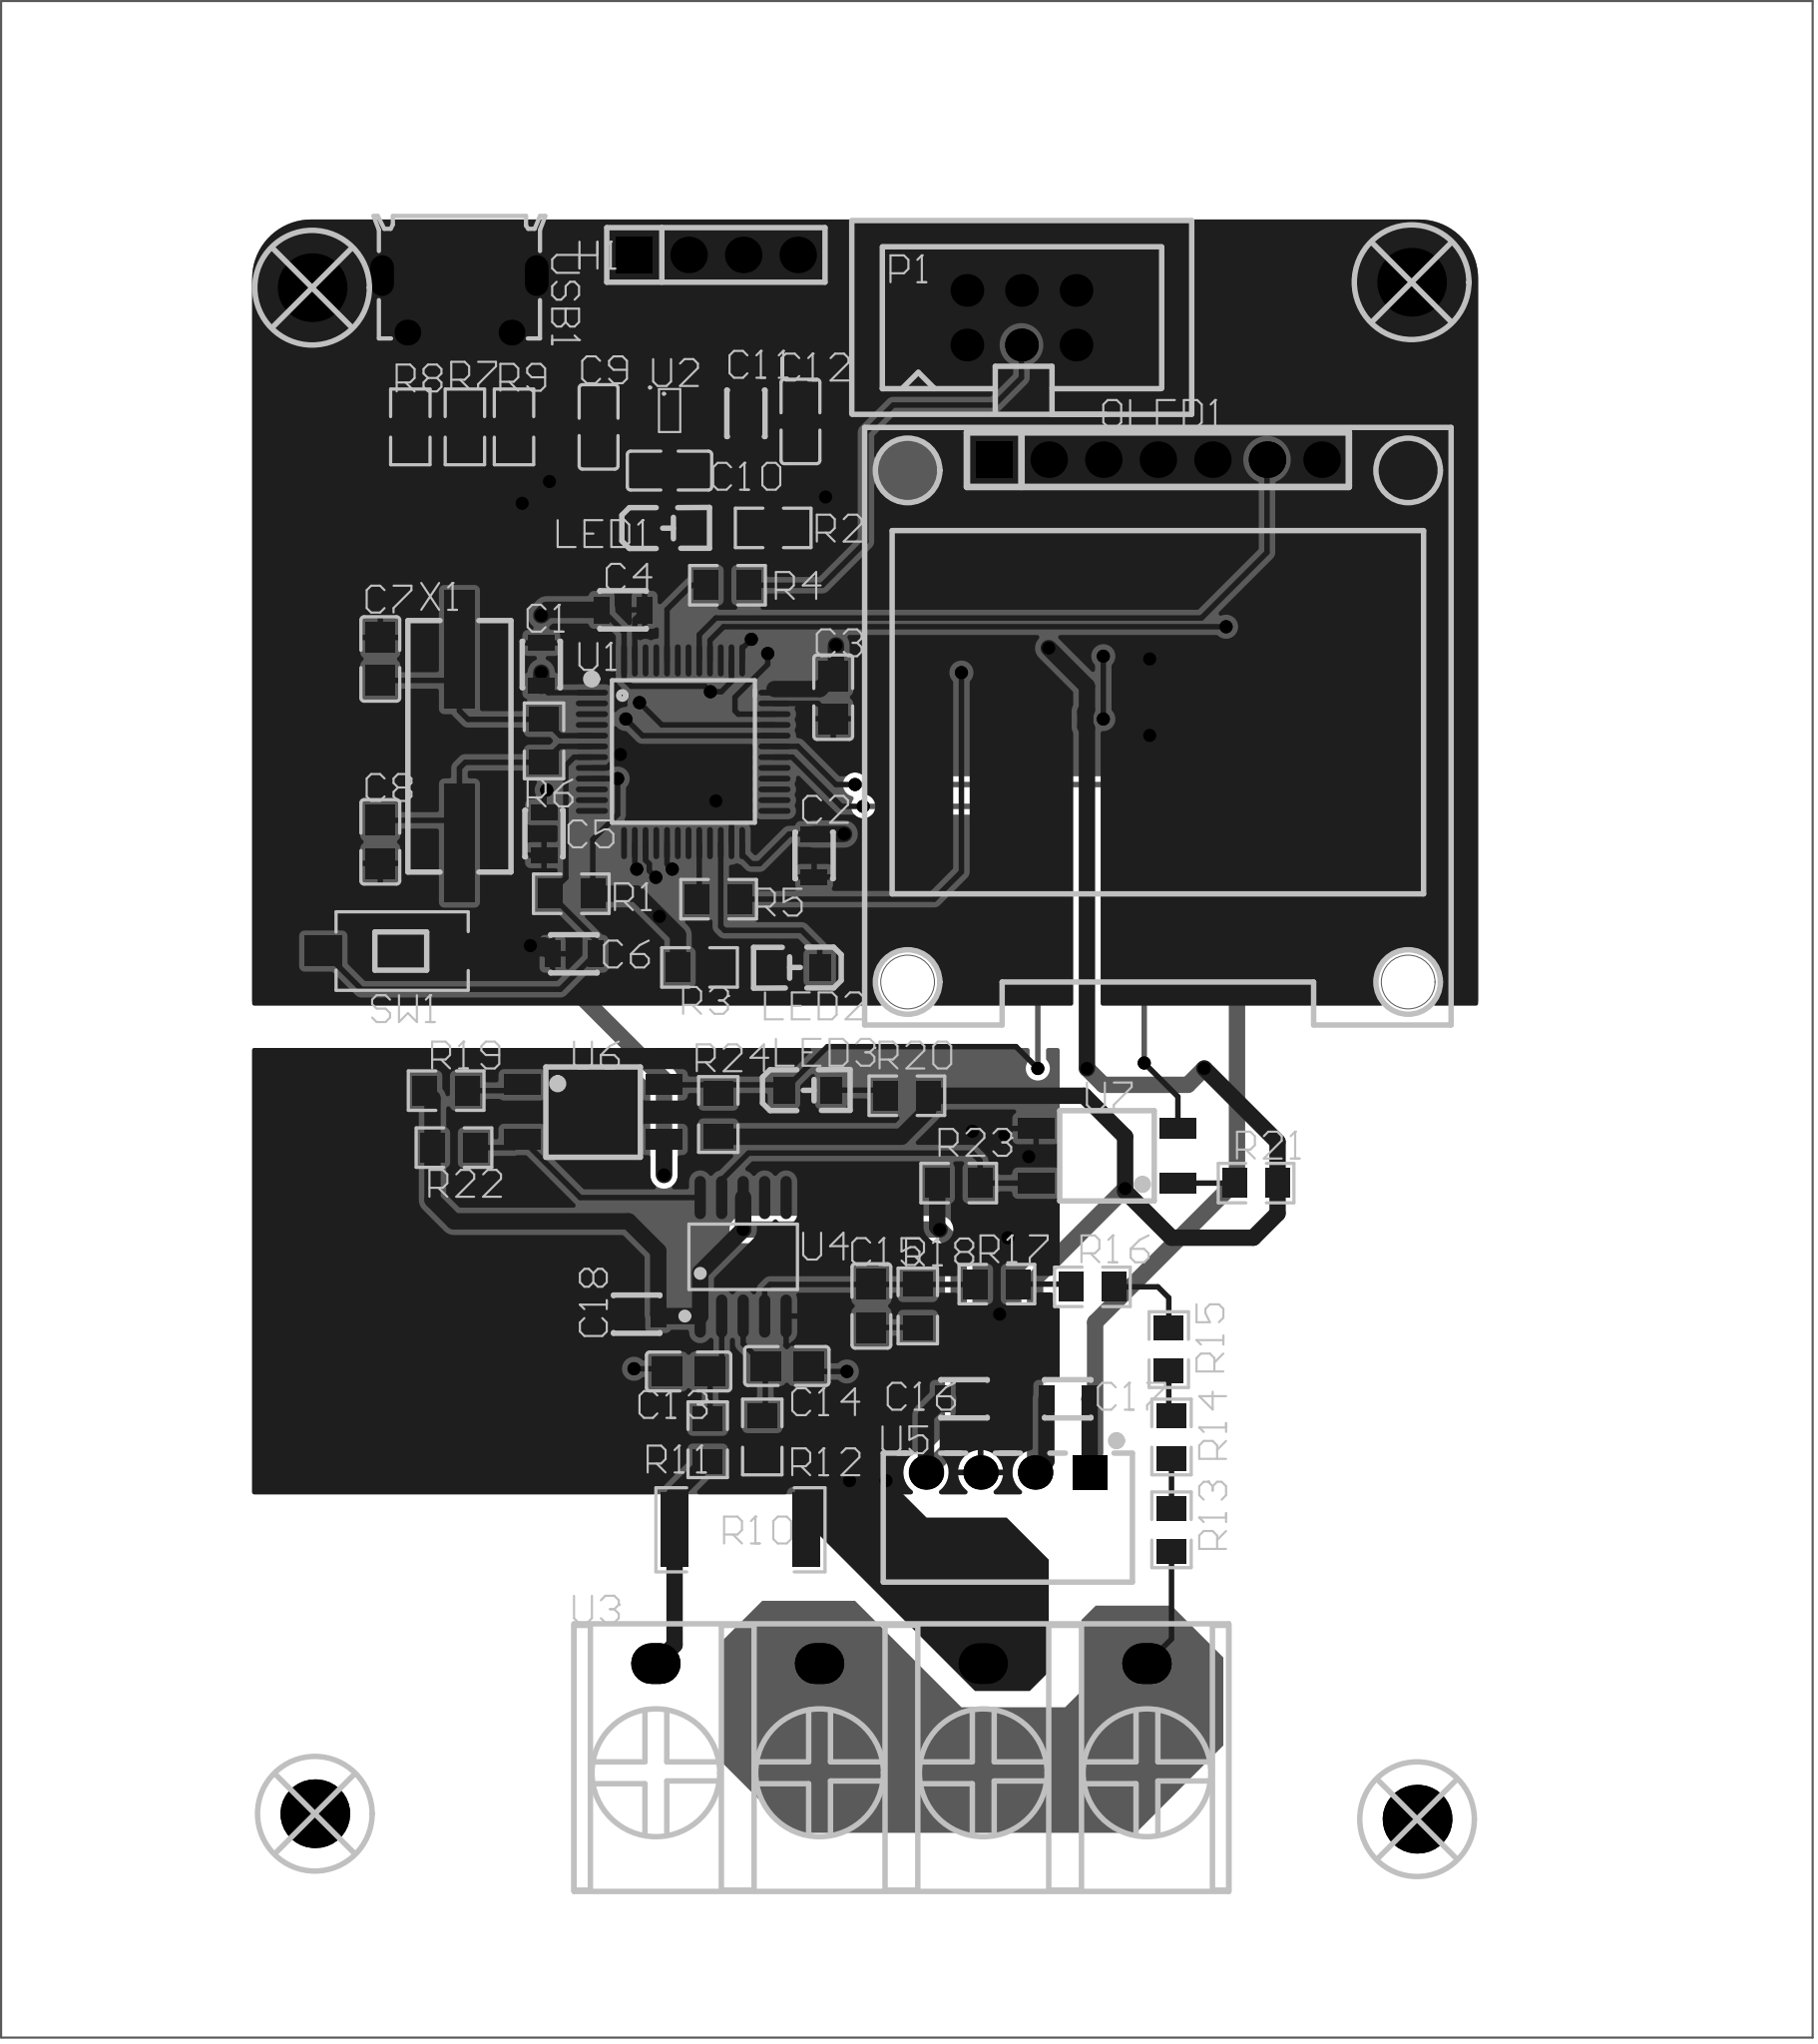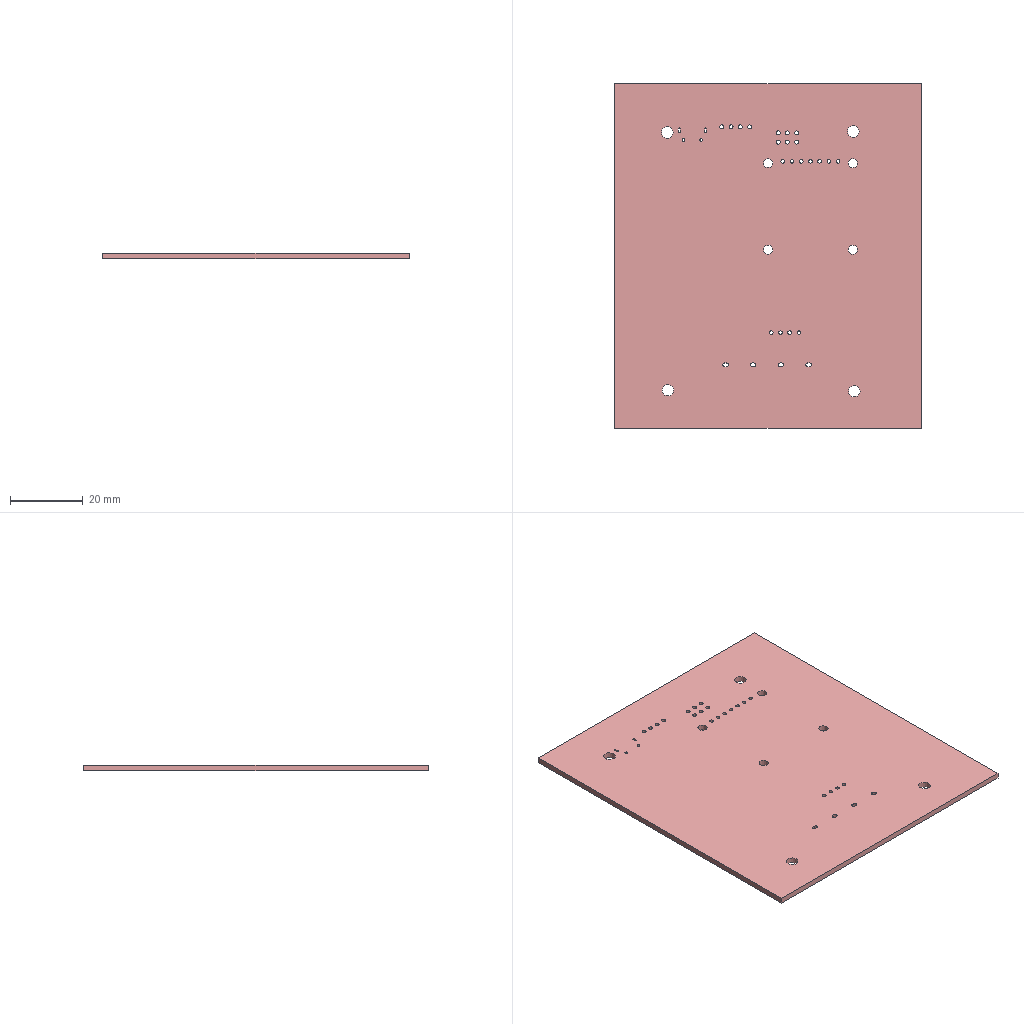Circuit board layout | Altium Designer | box 84.3 x 94.7 x 1.6 mm
Layer stack:
# Altium Designer layer stack of  (unit mm; dielectric type: 0 none, 1 core, 2 prepreg, 3 surface material)
index,name,kind,layer,copper_thickness_mm,dielectric_type,dielectric_thickness_mm,dielectric_material,dielectric_constant
0,Top Paste Mask Layer,other,,,,,,
1,Top Silkscreen Layer,other,,,,,,
2,Top Solder Mask Layer,dielectric,,,3,0.01,,3.3
3,Top Layer,copper,Top Layer,0.035,,,,
4,Dielectric1,dielectric,,,3,1.51,FR4,4.5
5,Bottom Layer,copper,Bottom Layer,0.035,,,,
6,Bottom Solder Mask Layer,dielectric,,,3,0.01,,3.3
7,Bottom Silkscreen Layer,other,,,,,,
8,Bottom Paste Mask Layer,other,,,,,,
# drill layer pairs: low layer,high layer
drill_pair,Top Layer,Bottom Layer
Part placement:
Designator,Comment,Layer,Footprint,Center-X(mm),Center-Y(mm),Rotation
C1,100nF,TopLayer,CAP-SMD_L2.0-W1.25,94.996,133.731,270
C2,100nF,TopLayer,CAP-SMD_L2.0-W1.25,107.696,124.841,90
C3,2.2uF,TopLayer,C0805,108.585,132.207,270
C4,100nF,TopLayer,CAP-SMD_L2.0-W1.25,98.806,136.271,180
C5,100nF,TopLayer,CAP-SMD_L2.0-W1.25,95.123,125.857,90
C6,100nF,TopLayer,CAP-SMD_L2.0-W1.25,96.52,120.269,180
C7,22pF,TopLayer,C0805,87.503,133.985,90
C8,22pF,TopLayer,C0805,87.503,125.476,270
C9,1uF,TopLayer,C0805,97.663,144.78,90
C10,22nF,TopLayer,C0805,100.965,142.748,0
C11,100nF,TopLayer,CAP-SMD_L2.0-W1.25,104.521,145.415,270
C12,10uF,TopLayer,C0805,107.061,145.034,90
C13,68nF,TopLayer,C0805,101.854,100.838,180
C14,68nF,TopLayer,C0805,106.426,101.092,180
C15,68nF,TopLayer,C0805,110.363,103.886,270
C16,100nF,TopLayer,CAP-SMD_L2.0-W1.25,114.681,99.568,180
C17,100nF,TopLayer,CAP-SMD_L2.0-W1.25,119.507,99.568,180
C18,100nF,TopLayer,CAP-SMD_L2.0-W1.25,99.441,103.505,180
H1,PZ254V-11-04P,TopLayer,HDR-TH_4P-P2.54-V-M,103.124,152.781,0
LED1,,TopLayer,LED_0805,100.847,140.074,0
LED2,,TopLayer,LED_0805,106.857,119.629,180
LED3,,TopLayer,LED_0805,107.392,113.924,0
OLED1,HS96L01W4S03,TopLayer,OLED-TH_HS96L01W4S03,123.698,143.256,0
P1,2.54-2*3P pin header,TopLayer,IDC-TH_6P-P2.54_C11214,117.348,149.86,0
R1,10kΩ,TopLayer,R0805,96.393,123.063,0
R2,1kΩ,TopLayer,R0805,105.791,140.081,0
R3,1kΩ,TopLayer,R0805,102.362,119.634,180
R4,10kΩ,TopLayer,R0805,103.664,137.414,180
R5,10kΩ,TopLayer,R0805,103.251,122.809,0
R6,1MΩ,TopLayer,R0805,95.123,130.175,90
R7,20Ω,TopLayer,R0805,91.44,144.78,270
R8,20Ω,TopLayer,R0805,88.9,144.78,270
R9,4.7kΩ,TopLayer,R0805,93.726,144.78,270
R10,3mΩ,TopLayer,R2512,104.267,93.472,180
R11,510Ω,TopLayer,R0805,102.743,97.663,270
R12,510Ω,TopLayer,R0805,105.283,97.79,270
R13,390kΩ,TopLayer,R0805,124.333,93.472,270
R14,390kΩ,TopLayer,R0805,124.333,97.79,270
R15,390kΩ,TopLayer,R0805,124.206,101.854,270
R16,390kΩ,TopLayer,R0805,120.65,104.775,0
R17,390kΩ,TopLayer,R0805,116.205,104.902,0
R18,510Ω,TopLayer,R0805,112.522,103.886,270
R19,1kΩ,TopLayer,R0805,90.567,113.903,180
R20,1kΩ,TopLayer,R0805,112.014,113.665,180
R21,1kΩ,TopLayer,R0805,128.27,109.601,0
R22,10kΩ,TopLayer,R0805,90.932,111.252,180
R23,10kΩ,TopLayer,R0805,114.427,109.601,180
R24,3.3kΩ,TopLayer,R0805,103.235,112.792,90
SW1,TS1305-TZ43HBM,TopLayer,SW-SMD_L6.0-W3.5-LS8.0_TS04-TBW1FH4.3,88.519,120.396,180
U1,STM32F103C8T6,TopLayer,LQFP-48_L7.0-W7.0-P0.50-LS9.0-BL,101.6,129.667,270
U2,RT9193-33GU5,TopLayer,SC-70-5_L2.0-W1.3-P0.65-LS2.1-BL,100.965,145.542,270
U3,DBT10-7.62-4P-GN-P,TopLayer,CONN-TH_DBT10-7.62-4P,111.76,87.249,0
U4,BL0942,TopLayer,SSOP-10_L4.9-W3.9-P1.00-LS6.0-BL,104.394,106.172,0
U5,B0303S-1W,TopLayer,PWRM-TH_BXXXXS-1W,116.713,96.139,180
U6,EL357N(C)(TA)-G,TopLayer,OPTO-SMD-4_L4.4-W4.1-P2.54-LS7.0-TL,97.409,112.903,0
U7,EL357N(C)(TA)-G,TopLayer,OPTO-SMD-4_L4.4-W4.1-P2.54-LS7.0-TL,121.33,110.871,180
USB1,920-E52A2021S10100,TopLayer,MICRO-USB-SMD_5P-P0.65-H-F_C10418,91.186,150.495,180
X1,8MHz,TopLayer,CRYSTAL-SMD_L11.4-W4.7-LS12.7,91.186,129.921,90
SCREW1,,TopLayer,M3螺丝,84.328,151.257,0
SCREW2,,TopLayer,M3螺丝,84.455,80.264,0
SCREW3,,TopLayer,M3螺丝,135.763,80.01,0
SCREW4,,TopLayer,M3螺丝,135.509,151.511,0
Pad and via stacks:
# Altium Designer via and pad stacks of  (unit mm). Each distinct definition once, with the count of objects using it.
# via: kind,start_layer,end_layer,hole_mm,diameter_mm,mode(0 simple;1 top-mid-bottom;2 full stack),diameter_per_layer,count,example_net
# pad: kind,layer,hole_mm,hole_type(0 round;1 square;2 slot),plating,top_size,top_shape(1 round;2 rect;3 octagon;9 rounded rect),mid_size,bottom_size,mode,footprint,size_per_layer,count,example
pad,Top Layer,0,0,plated,1.25x0.7,2,1.25x0.7,1.25x0.7,0,CAP-SMD_L2.0-W1.25,,18,C1.1
pad,Top Layer,0,0,plated,1.41x1.35,2,1.41x1.35,1.41x1.35,0,C0805,,18,C3.2
pad,Top Layer,0,0,plated,1x1.25,2,1x1.25,1x1.25,0,LED_0805,,6,LED1.2
pad,Top Layer,0,0,plated,1.133x1.377,2,1.133x1.377,1.133x1.377,0,R0805,,46,R1.2
pad,Top Layer,0,0,plated,1.282x3.456,2,1.282x3.456,1.282x3.456,0,R2512,,2,R10.2
pad,Top Layer,0,0,plated,1.74x1.4,2,1.74x1.4,1.74x1.4,0,SW-SMD_L6.0-W3.5-LS8.0_TS04-TBW1FH4.3,,2,SW1.1
pad,Top Layer,0,0,plated,0.27x1.5,1,0.27x1.5,0.27x1.5,0,LQFP-48_L7.0-W7.0-P0.50-LS9.0-BL,,24,U1.1
pad,Top Layer,0,0,plated,1.5x0.27,1,1.5x0.27,1.5x0.27,0,LQFP-48_L7.0-W7.0-P0.50-LS9.0-BL,,24,U1.13
pad,Top Layer,0,0,plated,0.35x0.85,2,0.35x0.85,0.35x0.85,0,SC-70-5_L2.0-W1.3-P0.65-LS2.1-BL,,5,U2.5
pad,Top Layer,0,0,plated,0.525x2.014,1,0.525x2.014,0.525x2.014,0,SSOP-10_L4.9-W3.9-P1.00-LS6.0-BL,,10,U4.1
pad,Top Layer,0,0,plated,1.7x0.95,2,1.7x0.95,1.7x0.95,0,OPTO-SMD-4_L4.4-W4.1-P2.54-LS7.0-TL,,8,U6.1
pad,Top Layer,0,0,plated,1.25x0.4,2,1.25x0.4,1.25x0.4,0,MICRO-USB-SMD_5P-P0.65-H-F_C10418,,5,USB1.5
pad,Top Layer,0,0,plated,5.5x1.4,2,5.5x1.4,5.5x1.4,0,CRYSTAL-SMD_L11.4-W4.7-LS12.7,,2,X1.2
pad,Multi-Layer,1.1,0,plated,1.7x1.7,2,1.7x1.7,1.7x1.7,0,HDR-TH_4P-P2.54-V-M,,1,H1.1
pad,Multi-Layer,1.1,0,plated,1.7x1.7,1,1.7x1.7,1.7x1.7,0,HDR-TH_4P-P2.54-V-M,,3,H1.2
pad,Multi-Layer,1,0,plated,1.7x1.7,1,1.7x1.7,1.7x1.7,0,OLED-TH_HS96L01W4S03,,6,OLED1.7
pad,Multi-Layer,1,0,plated,1.7x1.7,2,1.7x1.7,1.7x1.7,0,OLED-TH_HS96L01W4S03,,1,OLED1.1
pad,Multi-Layer,1.1,0,plated,1.524x1.524,1,1.524x1.524,1.524x1.524,0,IDC-TH_6P-P2.54_C11214,,6,P1.1
pad,Multi-Layer,1.1,2,plated,2.3x1.9,1,2.3x1.9,2.3x1.9,0,CONN-TH_DBT10-7.62-4P,,4,U3.1
pad,Multi-Layer,1,0,plated,1.6x1.6,2,1.6x1.6,1.6x1.6,0,PWRM-TH_BXXXXS-1W,,1,U5.1
pad,Multi-Layer,1,0,plated,1.6x1.6,1,1.6x1.6,1.6x1.6,0,PWRM-TH_BXXXXS-1W,,3,U5.2
pad,Multi-Layer,0.5,2,plated,1.1x1.9,1,1.1x1.9,1.1x1.9,0,MICRO-USB-SMD_5P-P0.65-H-F_C10418,,2,USB1.SH2
pad,Multi-Layer,0.7,0,plated,1.2x1.2,1,1.2x1.2,1.2x1.2,0,MICRO-USB-SMD_5P-P0.65-H-F_C10418,,2,USB1.SH0
pad,Multi-Layer,3.2,0,plated,3.2x3.2,1,3.2x3.2,3.2x3.2,0,M3\u00C2\u00DD\u00CB\u00BF,,4,SCREW1.1
via,Top Layer,Bottom Layer,0.3048,0.6096,0,,47,ORX
Copper pours:
name,layer,net,type(0 solid;1 hatched;2 none)
Bottom Layer-AGND,Bottom Layer,AGND,0
Bottom Layer-GND,Bottom Layer,GND,0
Top Layer-AGND,Top Layer,AGND,0
Top Layer-GND,Top Layer,GND,0
Design rules, without the lines most boards share:
# Altium Designer design rules of  (exported by Altium Designer, unit mm)
# columns: name | kind | enabled | priority | scope1 | scope2 | descriptor | typed fields (field=value)
safeClearance | 0 | enabled | 1 | All | All | Clearance Constraint (Gap=6mil) (All),(All) | gap=0.1524
safeClearance_1 | 63 | enabled | 1 | All | All | Board Clearance Constraint (Gap=0mil) (All) |
otherClearance | 52 | enabled | 1 | All | All | Hole To Hole Clearance (Gap=11.2mil) (All),(All) | gap=0.2845
power | 2 | enabled | 1 | (InNet('GND') OR InNet('VCC3.3') OR InNet('+5V') OR InNet('AGND') OR InNet('VCC')) | All | Width Constraint (Min=10mil) (Max=100mil) (Preferred=30mil) ((InNet('GND') OR InNet('VCC3.3') OR InNet('+5V') OR InNet('AGND') OR InNet('VCC'))) |
trackWidth | 2 | enabled | 2 | All | All | Width Constraint (Min=5mil) (Max=100mil) (Preferred=10mil) (All) |
viaSize | 11 | enabled | 1 | All | All | Routing Via (MinHoleWidth=11.8mil) (MaxHoleWidth=236.2mil) (PreferredHoleWidth=12mil) (MinWidth=19.7mil) (MaxWidth=393.7mil) (PreferedWidth=24mil) (All) | via_min_hole=0.2997 via_max_hole=6 via_preferred_diameter=0.6096 via_preferred_hole=0.3048
copperRegion | 20 | enabled | 1 | (InNet('GND') OR InNet('AGND')) | All | Polygon Connect Rule(Relief Connect )(Conductor Width=10mil) (Relief Angle=90 Angle) (Entries=4) (Air Gap Width=10mil) ((InNet('GND') OR InNet('AGND'))),(All) | connect_style(0=relief,1=direct,2=none)=0 relief_conductor_width=0.254 relief_entries=4